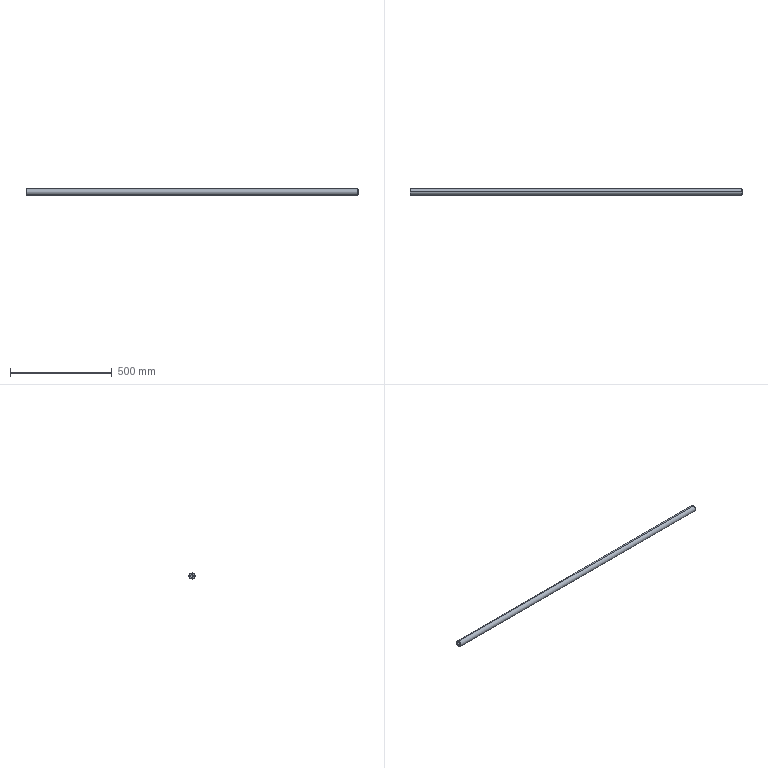Part | SolidWorks | features BaseBody 1 | 1 solid | 16 faces | box 1632 x 30 x 30 mm | volume 1142665 mm3 | cone 8 | cylinder 6 | plane 2 | commonest cylinder face diameters 14 x4 30 x2
STEP:
#1=CARTESIAN_POINT('',(-782.206,0.,-7.));
#2=VERTEX_POINT('',#1);
#3=CARTESIAN_POINT('',(-782.206,0.,7.));
#4=VERTEX_POINT('',#3);
#5=CARTESIAN_POINT('',(-782.206,0.,0.));
#6=DIRECTION('',(-1.,0.,0.));
#7=DIRECTION('',(0.,0.,1.));
#8=AXIS2_PLACEMENT_3D('',#5,#6,#7);
#9=CIRCLE('',#8,7.);
#10=EDGE_CURVE('',#2,#4,#9,.T.);
#11=ORIENTED_EDGE('',*,*,#10,.F.);
#12=CARTESIAN_POINT('',(-816.,0.,-7.));
#13=VERTEX_POINT('',#12);
#14=CARTESIAN_POINT('',(-816.,0.,-7.));
#15=DIRECTION('',(-1.,0.,0.));
#16=VECTOR('',#15,1000.);
#17=LINE('',#14,#16);
#18=EDGE_CURVE('',#2,#13,#17,.T.);
#19=ORIENTED_EDGE('',*,*,#18,.T.);
#20=CARTESIAN_POINT('',(-816.,0.,7.));
#21=VERTEX_POINT('',#20);
#22=CARTESIAN_POINT('',(-816.,0.,0.));
#23=DIRECTION('',(-1.,0.,0.));
#24=DIRECTION('',(0.,0.,1.));
#25=AXIS2_PLACEMENT_3D('',#22,#23,#24);
#26=CIRCLE('',#25,7.);
#27=EDGE_CURVE('',#13,#21,#26,.T.);
#28=ORIENTED_EDGE('',*,*,#27,.T.);
#29=CARTESIAN_POINT('',(-816.,0.,7.));
#30=DIRECTION('',(-1.,0.,0.));
#31=VECTOR('',#30,1000.);
#32=LINE('',#29,#31);
#33=EDGE_CURVE('',#4,#21,#32,.T.);
#34=ORIENTED_EDGE('',*,*,#33,.F.);
#35=EDGE_LOOP('',(#11,#19,#28,#34));
#36=FACE_OUTER_BOUND('',#35,.T.);
#37=CARTESIAN_POINT('',(-816.,0.,0.));
#38=DIRECTION('',(-1.,0.,0.));
#39=DIRECTION('',(0.,0.,1.));
#40=AXIS2_PLACEMENT_3D('',#37,#38,#39);
#41=CYLINDRICAL_SURFACE('',#40,7.);
#42=ADVANCED_FACE('',(#36),#41,.F.);
#43=CARTESIAN_POINT('',(-778.,0.,0.));
#44=VERTEX_POINT('',#43);
#45=CARTESIAN_POINT('',(-782.206,0.,7.));
#46=DIRECTION('',(-0.515,0.,0.8572));
#47=VECTOR('',#46,1000.);
#48=LINE('',#45,#47);
#49=EDGE_CURVE('',#44,#4,#48,.T.);
#50=ORIENTED_EDGE('',*,*,#49,.F.);
#51=CARTESIAN_POINT('',(-782.206,0.,-7.));
#52=DIRECTION('',(-0.515,0.,-0.8572));
#53=VECTOR('',#52,1000.);
#54=LINE('',#51,#53);
#55=EDGE_CURVE('',#44,#2,#54,.T.);
#56=ORIENTED_EDGE('',*,*,#55,.T.);
#57=ORIENTED_EDGE('',*,*,#10,.T.);
#58=EDGE_LOOP('',(#50,#56,#57));
#59=FACE_OUTER_BOUND('',#58,.T.);
#60=CARTESIAN_POINT('',(-782.206,0.,0.));
#61=DIRECTION('',(-1.,0.,0.));
#62=DIRECTION('',(0.,0.,1.));
#63=AXIS2_PLACEMENT_3D('',#60,#61,#62);
#64=CONICAL_SURFACE('',#63,7.,1.03);
#65=ADVANCED_FACE('',(#59),#64,.F.);
#66=CARTESIAN_POINT('',(782.206,0.,7.));
#67=VERTEX_POINT('',#66);
#68=CARTESIAN_POINT('',(782.206,0.,-7.));
#69=VERTEX_POINT('',#68);
#70=CARTESIAN_POINT('',(782.206,0.,0.));
#71=DIRECTION('',(1.,0.,0.));
#72=DIRECTION('',(0.,0.,-1.));
#73=AXIS2_PLACEMENT_3D('',#70,#71,#72);
#74=CIRCLE('',#73,7.);
#75=EDGE_CURVE('',#67,#69,#74,.T.);
#76=ORIENTED_EDGE('',*,*,#75,.F.);
#77=CARTESIAN_POINT('',(816.,0.,7.));
#78=VERTEX_POINT('',#77);
#79=CARTESIAN_POINT('',(816.,0.,7.));
#80=DIRECTION('',(1.,0.,0.));
#81=VECTOR('',#80,1000.);
#82=LINE('',#79,#81);
#83=EDGE_CURVE('',#67,#78,#82,.T.);
#84=ORIENTED_EDGE('',*,*,#83,.T.);
#85=CARTESIAN_POINT('',(816.,0.,-7.));
#86=VERTEX_POINT('',#85);
#87=CARTESIAN_POINT('',(816.,0.,0.));
#88=DIRECTION('',(1.,0.,0.));
#89=DIRECTION('',(0.,0.,-1.));
#90=AXIS2_PLACEMENT_3D('',#87,#88,#89);
#91=CIRCLE('',#90,7.);
#92=EDGE_CURVE('',#78,#86,#91,.T.);
#93=ORIENTED_EDGE('',*,*,#92,.T.);
#94=CARTESIAN_POINT('',(816.,0.,-7.));
#95=DIRECTION('',(1.,0.,0.));
#96=VECTOR('',#95,1000.);
#97=LINE('',#94,#96);
#98=EDGE_CURVE('',#69,#86,#97,.T.);
#99=ORIENTED_EDGE('',*,*,#98,.F.);
#100=EDGE_LOOP('',(#76,#84,#93,#99));
#101=FACE_OUTER_BOUND('',#100,.T.);
#102=CARTESIAN_POINT('',(816.,0.,0.));
#103=DIRECTION('',(1.,0.,0.));
#104=DIRECTION('',(0.,0.,-1.));
#105=AXIS2_PLACEMENT_3D('',#102,#103,#104);
#106=CYLINDRICAL_SURFACE('',#105,7.);
#107=ADVANCED_FACE('',(#101),#106,.F.);
#108=CARTESIAN_POINT('',(778.,0.,0.));
#109=VERTEX_POINT('',#108);
#110=CARTESIAN_POINT('',(782.206,0.,-7.));
#111=DIRECTION('',(0.515,0.,-0.8572));
#112=VECTOR('',#111,1000.);
#113=LINE('',#110,#112);
#114=EDGE_CURVE('',#109,#69,#113,.T.);
#115=ORIENTED_EDGE('',*,*,#114,.F.);
#116=CARTESIAN_POINT('',(782.206,0.,7.));
#117=DIRECTION('',(0.515,0.,0.8572));
#118=VECTOR('',#117,1000.);
#119=LINE('',#116,#118);
#120=EDGE_CURVE('',#109,#67,#119,.T.);
#121=ORIENTED_EDGE('',*,*,#120,.T.);
#122=ORIENTED_EDGE('',*,*,#75,.T.);
#123=EDGE_LOOP('',(#115,#121,#122));
#124=FACE_OUTER_BOUND('',#123,.T.);
#125=CARTESIAN_POINT('',(782.206,0.,0.));
#126=DIRECTION('',(1.,0.,0.));
#127=DIRECTION('',(0.,0.,-1.));
#128=AXIS2_PLACEMENT_3D('',#125,#126,#127);
#129=CONICAL_SURFACE('',#128,7.,1.03);
#130=ADVANCED_FACE('',(#124),#129,.F.);
#131=CARTESIAN_POINT('',(816.,0.,-14.));
#132=VERTEX_POINT('',#131);
#133=CARTESIAN_POINT('',(816.,0.,14.));
#134=VERTEX_POINT('',#133);
#135=CARTESIAN_POINT('',(816.,0.,0.));
#136=DIRECTION('',(1.,0.,0.));
#137=DIRECTION('',(0.,0.,-1.));
#138=AXIS2_PLACEMENT_3D('',#135,#136,#137);
#139=CIRCLE('',#138,14.);
#140=EDGE_CURVE('',#132,#134,#139,.T.);
#141=ORIENTED_EDGE('',*,*,#140,.F.);
#142=CARTESIAN_POINT('',(815.,0.,-15.));
#143=VERTEX_POINT('',#142);
#144=CARTESIAN_POINT('',(816.,0.,-14.));
#145=DIRECTION('',(-0.7071,0.,-0.7071));
#146=VECTOR('',#145,1000.);
#147=LINE('',#144,#146);
#148=EDGE_CURVE('',#132,#143,#147,.T.);
#149=ORIENTED_EDGE('',*,*,#148,.T.);
#150=CARTESIAN_POINT('',(815.,0.,15.));
#151=VERTEX_POINT('',#150);
#152=CARTESIAN_POINT('',(815.,0.,0.));
#153=DIRECTION('',(-1.,0.,0.));
#154=DIRECTION('',(0.,0.,-1.));
#155=AXIS2_PLACEMENT_3D('',#152,#153,#154);
#156=CIRCLE('',#155,15.);
#157=EDGE_CURVE('',#151,#143,#156,.T.);
#158=ORIENTED_EDGE('',*,*,#157,.F.);
#159=CARTESIAN_POINT('',(816.,0.,14.));
#160=DIRECTION('',(-0.7071,0.,0.7071));
#161=VECTOR('',#160,1000.);
#162=LINE('',#159,#161);
#163=EDGE_CURVE('',#134,#151,#162,.T.);
#164=ORIENTED_EDGE('',*,*,#163,.F.);
#165=EDGE_LOOP('',(#141,#149,#158,#164));
#166=FACE_OUTER_BOUND('',#165,.T.);
#167=CARTESIAN_POINT('',(816.,0.,0.));
#168=DIRECTION('',(-1.,0.,0.));
#169=DIRECTION('',(0.,0.,1.));
#170=AXIS2_PLACEMENT_3D('',#167,#168,#169);
#171=CONICAL_SURFACE('',#170,14.,0.7854);
#172=ADVANCED_FACE('',(#166),#171,.T.);
#173=CARTESIAN_POINT('',(-816.,0.,14.));
#174=VERTEX_POINT('',#173);
#175=CARTESIAN_POINT('',(-816.,0.,-14.));
#176=VERTEX_POINT('',#175);
#177=CARTESIAN_POINT('',(-816.,0.,0.));
#178=DIRECTION('',(-1.,0.,0.));
#179=DIRECTION('',(0.,0.,-1.));
#180=AXIS2_PLACEMENT_3D('',#177,#178,#179);
#181=CIRCLE('',#180,14.);
#182=EDGE_CURVE('',#174,#176,#181,.T.);
#183=ORIENTED_EDGE('',*,*,#182,.F.);
#184=CARTESIAN_POINT('',(-815.,0.,15.));
#185=VERTEX_POINT('',#184);
#186=CARTESIAN_POINT('',(-815.,0.,15.));
#187=DIRECTION('',(0.7071,0.,0.7071));
#188=VECTOR('',#187,1000.);
#189=LINE('',#186,#188);
#190=EDGE_CURVE('',#174,#185,#189,.T.);
#191=ORIENTED_EDGE('',*,*,#190,.T.);
#192=CARTESIAN_POINT('',(-815.,0.,-15.));
#193=VERTEX_POINT('',#192);
#194=CARTESIAN_POINT('',(-815.,0.,0.));
#195=DIRECTION('',(1.,0.,0.));
#196=DIRECTION('',(0.,0.,-1.));
#197=AXIS2_PLACEMENT_3D('',#194,#195,#196);
#198=CIRCLE('',#197,15.);
#199=EDGE_CURVE('',#193,#185,#198,.T.);
#200=ORIENTED_EDGE('',*,*,#199,.F.);
#201=CARTESIAN_POINT('',(-815.,0.,-15.));
#202=DIRECTION('',(0.7071,0.,-0.7071));
#203=VECTOR('',#202,1000.);
#204=LINE('',#201,#203);
#205=EDGE_CURVE('',#176,#193,#204,.T.);
#206=ORIENTED_EDGE('',*,*,#205,.F.);
#207=EDGE_LOOP('',(#183,#191,#200,#206));
#208=FACE_OUTER_BOUND('',#207,.T.);
#209=CARTESIAN_POINT('',(-815.,0.,0.));
#210=DIRECTION('',(1.,0.,0.));
#211=DIRECTION('',(0.,0.,-1.));
#212=AXIS2_PLACEMENT_3D('',#209,#210,#211);
#213=CONICAL_SURFACE('',#212,15.,0.7854);
#214=ADVANCED_FACE('',(#208),#213,.T.);
#215=ORIENTED_EDGE('',*,*,#157,.T.);
#216=CARTESIAN_POINT('',(816.,0.,-15.));
#217=DIRECTION('',(-1.,0.,0.));
#218=VECTOR('',#217,1000.);
#219=LINE('',#216,#218);
#220=EDGE_CURVE('',#143,#193,#219,.T.);
#221=ORIENTED_EDGE('',*,*,#220,.T.);
#222=ORIENTED_EDGE('',*,*,#199,.T.);
#223=CARTESIAN_POINT('',(816.,0.,15.));
#224=DIRECTION('',(-1.,0.,0.));
#225=VECTOR('',#224,1000.);
#226=LINE('',#223,#225);
#227=EDGE_CURVE('',#151,#185,#226,.T.);
#228=ORIENTED_EDGE('',*,*,#227,.F.);
#229=EDGE_LOOP('',(#215,#221,#222,#228));
#230=FACE_OUTER_BOUND('',#229,.T.);
#231=CARTESIAN_POINT('',(816.,0.,0.));
#232=DIRECTION('',(-1.,0.,0.));
#233=DIRECTION('',(0.,0.,1.));
#234=AXIS2_PLACEMENT_3D('',#231,#232,#233);
#235=CYLINDRICAL_SURFACE('',#234,15.);
#236=ADVANCED_FACE('',(#230),#235,.T.);
#237=ORIENTED_EDGE('',*,*,#220,.F.);
#238=CARTESIAN_POINT('',(815.,0.,0.));
#239=DIRECTION('',(-1.,0.,0.));
#240=DIRECTION('',(0.,0.,-1.));
#241=AXIS2_PLACEMENT_3D('',#238,#239,#240);
#242=CIRCLE('',#241,15.);
#243=EDGE_CURVE('',#143,#151,#242,.T.);
#244=ORIENTED_EDGE('',*,*,#243,.T.);
#245=ORIENTED_EDGE('',*,*,#227,.T.);
#246=CARTESIAN_POINT('',(-815.,0.,0.));
#247=DIRECTION('',(1.,0.,0.));
#248=DIRECTION('',(0.,0.,-1.));
#249=AXIS2_PLACEMENT_3D('',#246,#247,#248);
#250=CIRCLE('',#249,15.);
#251=EDGE_CURVE('',#185,#193,#250,.T.);
#252=ORIENTED_EDGE('',*,*,#251,.T.);
#253=EDGE_LOOP('',(#237,#244,#245,#252));
#254=FACE_OUTER_BOUND('',#253,.T.);
#255=CARTESIAN_POINT('',(816.,0.,0.));
#256=DIRECTION('',(-1.,0.,0.));
#257=DIRECTION('',(0.,0.,1.));
#258=AXIS2_PLACEMENT_3D('',#255,#256,#257);
#259=CYLINDRICAL_SURFACE('',#258,15.);
#260=ADVANCED_FACE('',(#254),#259,.T.);
#261=CARTESIAN_POINT('',(816.,0.,0.));
#262=DIRECTION('',(1.,0.,0.));
#263=DIRECTION('',(0.,0.,-1.));
#264=AXIS2_PLACEMENT_3D('',#261,#262,#263);
#265=CIRCLE('',#264,7.);
#266=EDGE_CURVE('',#86,#78,#265,.T.);
#267=ORIENTED_EDGE('',*,*,#266,.F.);
#268=ORIENTED_EDGE('',*,*,#92,.F.);
#269=EDGE_LOOP('',(#267,#268));
#270=FACE_BOUND('',#269,.T.);
#271=CARTESIAN_POINT('',(816.,0.,0.));
#272=DIRECTION('',(1.,0.,0.));
#273=DIRECTION('',(0.,0.,-1.));
#274=AXIS2_PLACEMENT_3D('',#271,#272,#273);
#275=CIRCLE('',#274,14.);
#276=EDGE_CURVE('',#134,#132,#275,.T.);
#277=ORIENTED_EDGE('',*,*,#276,.T.);
#278=ORIENTED_EDGE('',*,*,#140,.T.);
#279=EDGE_LOOP('',(#277,#278));
#280=FACE_OUTER_BOUND('',#279,.T.);
#281=CARTESIAN_POINT('',(816.,0.,0.));
#282=DIRECTION('',(1.,0.,0.));
#283=DIRECTION('',(0.,0.,-1.));
#284=AXIS2_PLACEMENT_3D('',#281,#282,#283);
#285=PLANE('',#284);
#286=ADVANCED_FACE('',(#270,#280),#285,.T.);
#287=CARTESIAN_POINT('',(-816.,0.,0.));
#288=DIRECTION('',(-1.,0.,0.));
#289=DIRECTION('',(0.,0.,1.));
#290=AXIS2_PLACEMENT_3D('',#287,#288,#289);
#291=CIRCLE('',#290,7.);
#292=EDGE_CURVE('',#21,#13,#291,.T.);
#293=ORIENTED_EDGE('',*,*,#292,.F.);
#294=ORIENTED_EDGE('',*,*,#27,.F.);
#295=EDGE_LOOP('',(#293,#294));
#296=FACE_BOUND('',#295,.T.);
#297=CARTESIAN_POINT('',(-816.,0.,0.));
#298=DIRECTION('',(-1.,0.,0.));
#299=DIRECTION('',(0.,0.,-1.));
#300=AXIS2_PLACEMENT_3D('',#297,#298,#299);
#301=CIRCLE('',#300,14.);
#302=EDGE_CURVE('',#176,#174,#301,.T.);
#303=ORIENTED_EDGE('',*,*,#302,.T.);
#304=ORIENTED_EDGE('',*,*,#182,.T.);
#305=EDGE_LOOP('',(#303,#304));
#306=FACE_OUTER_BOUND('',#305,.T.);
#307=CARTESIAN_POINT('',(-816.,0.,0.));
#308=DIRECTION('',(1.,0.,0.));
#309=DIRECTION('',(0.,0.,-1.));
#310=AXIS2_PLACEMENT_3D('',#307,#308,#309);
#311=PLANE('',#310);
#312=ADVANCED_FACE('',(#296,#306),#311,.F.);
#313=ORIENTED_EDGE('',*,*,#190,.F.);
#314=ORIENTED_EDGE('',*,*,#302,.F.);
#315=ORIENTED_EDGE('',*,*,#205,.T.);
#316=ORIENTED_EDGE('',*,*,#251,.F.);
#317=EDGE_LOOP('',(#313,#314,#315,#316));
#318=FACE_OUTER_BOUND('',#317,.T.);
#319=CARTESIAN_POINT('',(-815.,0.,0.));
#320=DIRECTION('',(1.,0.,0.));
#321=DIRECTION('',(0.,0.,-1.));
#322=AXIS2_PLACEMENT_3D('',#319,#320,#321);
#323=CONICAL_SURFACE('',#322,15.,0.7854);
#324=ADVANCED_FACE('',(#318),#323,.T.);
#325=ORIENTED_EDGE('',*,*,#148,.F.);
#326=ORIENTED_EDGE('',*,*,#276,.F.);
#327=ORIENTED_EDGE('',*,*,#163,.T.);
#328=ORIENTED_EDGE('',*,*,#243,.F.);
#329=EDGE_LOOP('',(#325,#326,#327,#328));
#330=FACE_OUTER_BOUND('',#329,.T.);
#331=CARTESIAN_POINT('',(816.,0.,0.));
#332=DIRECTION('',(-1.,0.,0.));
#333=DIRECTION('',(0.,0.,1.));
#334=AXIS2_PLACEMENT_3D('',#331,#332,#333);
#335=CONICAL_SURFACE('',#334,14.,0.7854);
#336=ADVANCED_FACE('',(#330),#335,.T.);
#337=ORIENTED_EDGE('',*,*,#120,.F.);
#338=ORIENTED_EDGE('',*,*,#114,.T.);
#339=CARTESIAN_POINT('',(782.206,0.,0.));
#340=DIRECTION('',(1.,0.,0.));
#341=DIRECTION('',(0.,0.,-1.));
#342=AXIS2_PLACEMENT_3D('',#339,#340,#341);
#343=CIRCLE('',#342,7.);
#344=EDGE_CURVE('',#69,#67,#343,.T.);
#345=ORIENTED_EDGE('',*,*,#344,.T.);
#346=EDGE_LOOP('',(#337,#338,#345));
#347=FACE_OUTER_BOUND('',#346,.T.);
#348=CARTESIAN_POINT('',(782.206,0.,0.));
#349=DIRECTION('',(1.,0.,0.));
#350=DIRECTION('',(0.,0.,-1.));
#351=AXIS2_PLACEMENT_3D('',#348,#349,#350);
#352=CONICAL_SURFACE('',#351,7.,1.03);
#353=ADVANCED_FACE('',(#347),#352,.F.);
#354=ORIENTED_EDGE('',*,*,#83,.F.);
#355=ORIENTED_EDGE('',*,*,#344,.F.);
#356=ORIENTED_EDGE('',*,*,#98,.T.);
#357=ORIENTED_EDGE('',*,*,#266,.T.);
#358=EDGE_LOOP('',(#354,#355,#356,#357));
#359=FACE_OUTER_BOUND('',#358,.T.);
#360=CARTESIAN_POINT('',(816.,0.,0.));
#361=DIRECTION('',(1.,0.,0.));
#362=DIRECTION('',(0.,0.,-1.));
#363=AXIS2_PLACEMENT_3D('',#360,#361,#362);
#364=CYLINDRICAL_SURFACE('',#363,7.);
#365=ADVANCED_FACE('',(#359),#364,.F.);
#366=ORIENTED_EDGE('',*,*,#55,.F.);
#367=ORIENTED_EDGE('',*,*,#49,.T.);
#368=CARTESIAN_POINT('',(-782.206,0.,0.));
#369=DIRECTION('',(-1.,0.,0.));
#370=DIRECTION('',(0.,0.,1.));
#371=AXIS2_PLACEMENT_3D('',#368,#369,#370);
#372=CIRCLE('',#371,7.);
#373=EDGE_CURVE('',#4,#2,#372,.T.);
#374=ORIENTED_EDGE('',*,*,#373,.T.);
#375=EDGE_LOOP('',(#366,#367,#374));
#376=FACE_OUTER_BOUND('',#375,.T.);
#377=CARTESIAN_POINT('',(-782.206,0.,0.));
#378=DIRECTION('',(-1.,0.,0.));
#379=DIRECTION('',(0.,0.,1.));
#380=AXIS2_PLACEMENT_3D('',#377,#378,#379);
#381=CONICAL_SURFACE('',#380,7.,1.03);
#382=ADVANCED_FACE('',(#376),#381,.F.);
#383=ORIENTED_EDGE('',*,*,#18,.F.);
#384=ORIENTED_EDGE('',*,*,#373,.F.);
#385=ORIENTED_EDGE('',*,*,#33,.T.);
#386=ORIENTED_EDGE('',*,*,#292,.T.);
#387=EDGE_LOOP('',(#383,#384,#385,#386));
#388=FACE_OUTER_BOUND('',#387,.T.);
#389=CARTESIAN_POINT('',(-816.,0.,0.));
#390=DIRECTION('',(-1.,0.,0.));
#391=DIRECTION('',(0.,0.,1.));
#392=AXIS2_PLACEMENT_3D('',#389,#390,#391);
#393=CYLINDRICAL_SURFACE('',#392,7.);
#394=ADVANCED_FACE('',(#388),#393,.F.);
#395=CLOSED_SHELL('',(#42,#65,#107,#130,#172,#214,#236,#260,#286,#312,#324,#336,#353,#365,#382,#394));
#396=MANIFOLD_SOLID_BREP('',#395);
#397=CARTESIAN_POINT('',(0.,0.,0.));
#398=DIRECTION('',(0.,0.,1.));
#399=DIRECTION('',(1.,0.,0.));
#400=AXIS2_PLACEMENT_3D('',#397,#398,#399);
#401=(LENGTH_UNIT()NAMED_UNIT(*)SI_UNIT(.MILLI.,.METRE.));
#402=UNCERTAINTY_MEASURE_WITH_UNIT(LENGTH_MEASURE(0.00001),#401,'','');
#403=(NAMED_UNIT(*)PLANE_ANGLE_UNIT()SI_UNIT($,.RADIAN.));
#404=(NAMED_UNIT(*)SI_UNIT($,.STERADIAN.)SOLID_ANGLE_UNIT());
#405=(GEOMETRIC_REPRESENTATION_CONTEXT(3)GLOBAL_UNCERTAINTY_ASSIGNED_CONTEXT((#402))GLOBAL_UNIT_ASSIGNED_CONTEXT((#401,#403,#404))REPRESENTATION_CONTEXT('',''));
#406=ADVANCED_BREP_SHAPE_REPRESENTATION('',(#396,#400),#405);